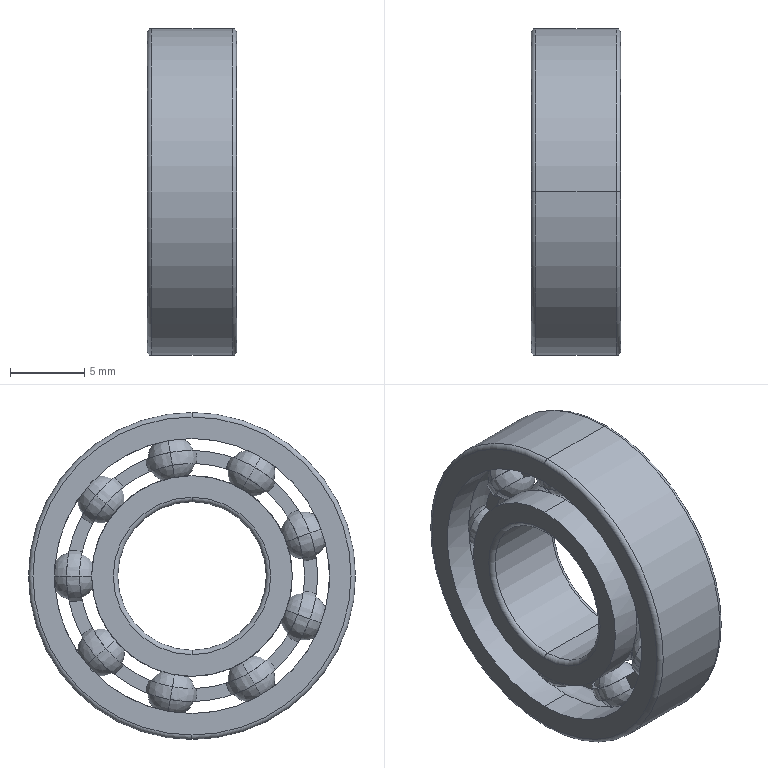Part | SolidWorks | features Revolution 5, CirPattern 2, RevCut 2 | 1 solid | 148 faces | box 6 x 22 x 22 mm | volume 1184 mm3 | sphere 72 | torus 38 | plane 22 | cylinder 16 | commonest cylinder face diameters 13.5 x4 18.5 x4 10 x2 15.127 x2 16.873 x2 22 x2